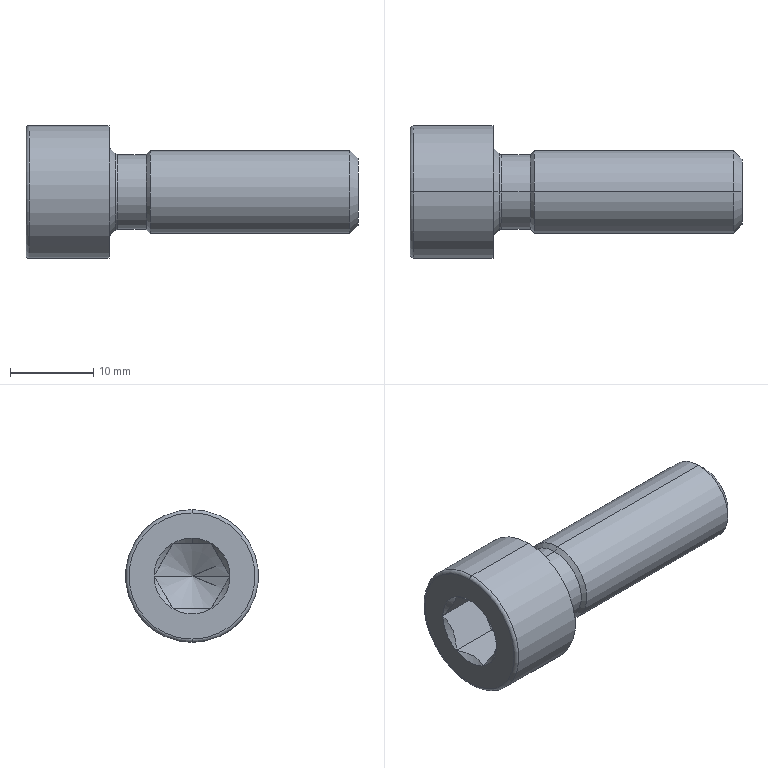Part | SolidWorks | features RevCut 2, Revolution 2, Chamfer 1, Cut 1, Fillet 1 | 1 solid | 42 faces | box 40 x 16 x 16 mm | volume 3907 mm3 | cone 15 | plane 15 | torus 6 | cylinder 6 | commonest cylinder face diameters 9.026 x2 10 x2 16 x2
STEP:
#1=CARTESIAN_POINT('',(40.,0.,-4.));
#2=VERTEX_POINT('',#1);
#3=CARTESIAN_POINT('',(40.,0.,4.));
#4=VERTEX_POINT('',#3);
#5=CARTESIAN_POINT('',(40.,0.,0.));
#6=DIRECTION('',(1.,0.,0.));
#7=DIRECTION('',(0.,0.,-1.));
#8=AXIS2_PLACEMENT_3D('',#5,#6,#7);
#9=CIRCLE('',#8,4.);
#10=EDGE_CURVE('',#2,#4,#9,.T.);
#11=ORIENTED_EDGE('',*,*,#10,.F.);
#12=CARTESIAN_POINT('',(39.,0.,-5.));
#13=VERTEX_POINT('',#12);
#14=CARTESIAN_POINT('',(40.,0.,-4.));
#15=DIRECTION('',(-0.7071,0.,-0.7071));
#16=VECTOR('',#15,1000.);
#17=LINE('',#14,#16);
#18=EDGE_CURVE('',#2,#13,#17,.T.);
#19=ORIENTED_EDGE('',*,*,#18,.T.);
#20=CARTESIAN_POINT('',(39.,0.,5.));
#21=VERTEX_POINT('',#20);
#22=CARTESIAN_POINT('',(39.,0.,0.));
#23=DIRECTION('',(-1.,0.,0.));
#24=DIRECTION('',(0.,0.,-1.));
#25=AXIS2_PLACEMENT_3D('',#22,#23,#24);
#26=CIRCLE('',#25,5.);
#27=EDGE_CURVE('',#21,#13,#26,.T.);
#28=ORIENTED_EDGE('',*,*,#27,.F.);
#29=CARTESIAN_POINT('',(40.,0.,4.));
#30=DIRECTION('',(-0.7071,0.,0.7071));
#31=VECTOR('',#30,1000.);
#32=LINE('',#29,#31);
#33=EDGE_CURVE('',#4,#21,#32,.T.);
#34=ORIENTED_EDGE('',*,*,#33,.F.);
#35=EDGE_LOOP('',(#11,#19,#28,#34));
#36=FACE_OUTER_BOUND('',#35,.T.);
#37=CARTESIAN_POINT('',(40.,0.,0.));
#38=DIRECTION('',(-1.,0.,0.));
#39=DIRECTION('',(0.,0.,1.));
#40=AXIS2_PLACEMENT_3D('',#37,#38,#39);
#41=CONICAL_SURFACE('',#40,4.,0.7854);
#42=ADVANCED_FACE('',(#36),#41,.T.);
#43=CARTESIAN_POINT('',(0.4,0.,-8.));
#44=VERTEX_POINT('',#43);
#45=CARTESIAN_POINT('',(0.4,0.,8.));
#46=VERTEX_POINT('',#45);
#47=CARTESIAN_POINT('',(0.4,0.,0.));
#48=DIRECTION('',(1.,0.,0.));
#49=DIRECTION('',(0.,0.,1.));
#50=AXIS2_PLACEMENT_3D('',#47,#48,#49);
#51=CIRCLE('',#50,8.);
#52=EDGE_CURVE('',#44,#46,#51,.T.);
#53=ORIENTED_EDGE('',*,*,#52,.F.);
#54=CARTESIAN_POINT('',(0.,0.,-7.6));
#55=VERTEX_POINT('',#54);
#56=CARTESIAN_POINT('',(0.4,0.,-7.6));
#57=DIRECTION('',(0.,1.,0.));
#58=DIRECTION('',(0.,0.,1.));
#59=AXIS2_PLACEMENT_3D('',#56,#57,#58);
#60=CIRCLE('',#59,0.4);
#61=EDGE_CURVE('',#44,#55,#60,.T.);
#62=ORIENTED_EDGE('',*,*,#61,.T.);
#63=CARTESIAN_POINT('',(0.,0.,7.6));
#64=VERTEX_POINT('',#63);
#65=CARTESIAN_POINT('',(0.,0.,0.));
#66=DIRECTION('',(-1.,0.,0.));
#67=DIRECTION('',(0.,0.,1.));
#68=AXIS2_PLACEMENT_3D('',#65,#66,#67);
#69=CIRCLE('',#68,7.6);
#70=EDGE_CURVE('',#64,#55,#69,.T.);
#71=ORIENTED_EDGE('',*,*,#70,.F.);
#72=CARTESIAN_POINT('',(0.4,0.,7.6));
#73=DIRECTION('',(0.,-1.,0.));
#74=DIRECTION('',(0.,0.,-1.));
#75=AXIS2_PLACEMENT_3D('',#72,#73,#74);
#76=CIRCLE('',#75,0.4);
#77=EDGE_CURVE('',#46,#64,#76,.T.);
#78=ORIENTED_EDGE('',*,*,#77,.F.);
#79=EDGE_LOOP('',(#53,#62,#71,#78));
#80=FACE_OUTER_BOUND('',#79,.T.);
#81=CARTESIAN_POINT('',(0.4,0.,0.));
#82=DIRECTION('',(-1.,0.,0.));
#83=DIRECTION('',(0.,0.,1.));
#84=AXIS2_PLACEMENT_3D('',#81,#82,#83);
#85=TOROIDAL_SURFACE('',#84,7.6,0.4);
#86=ADVANCED_FACE('',(#80),#85,.T.);
#87=CARTESIAN_POINT('',(8.641,0.,0.));
#88=VERTEX_POINT('',#87);
#89=CARTESIAN_POINT('',(6.,-4.575,0.));
#90=VERTEX_POINT('',#89);
#91=CARTESIAN_POINT('',(8.641,0.,0.));
#92=DIRECTION('',(-0.5,-0.866,0.));
#93=VECTOR('',#92,1000.);
#94=LINE('',#91,#93);
#95=EDGE_CURVE('',#88,#90,#94,.T.);
#96=ORIENTED_EDGE('',*,*,#95,.F.);
#97=CARTESIAN_POINT('',(6.,4.575,0.));
#98=VERTEX_POINT('',#97);
#99=CARTESIAN_POINT('',(8.641,0.,0.));
#100=DIRECTION('',(-0.5,0.866,0.));
#101=VECTOR('',#100,1000.);
#102=LINE('',#99,#101);
#103=EDGE_CURVE('',#88,#98,#102,.T.);
#104=ORIENTED_EDGE('',*,*,#103,.T.);
#105=CARTESIAN_POINT('',(6.,2.287,-3.962));
#106=VERTEX_POINT('',#105);
#107=CARTESIAN_POINT('',(6.,0.,0.));
#108=DIRECTION('',(-1.,0.,0.));
#109=DIRECTION('',(0.,-1.,0.));
#110=AXIS2_PLACEMENT_3D('',#107,#108,#109);
#111=CIRCLE('',#110,4.575);
#112=EDGE_CURVE('',#98,#106,#111,.T.);
#113=ORIENTED_EDGE('',*,*,#112,.T.);
#114=CARTESIAN_POINT('',(6.,-2.287,-3.962));
#115=VERTEX_POINT('',#114);
#116=CARTESIAN_POINT('',(6.,0.,0.));
#117=DIRECTION('',(-1.,0.,0.));
#118=DIRECTION('',(0.,-1.,0.));
#119=AXIS2_PLACEMENT_3D('',#116,#117,#118);
#120=CIRCLE('',#119,4.575);
#121=EDGE_CURVE('',#106,#115,#120,.T.);
#122=ORIENTED_EDGE('',*,*,#121,.T.);
#123=CARTESIAN_POINT('',(6.,0.,0.));
#124=DIRECTION('',(-1.,0.,0.));
#125=DIRECTION('',(0.,-1.,0.));
#126=AXIS2_PLACEMENT_3D('',#123,#124,#125);
#127=CIRCLE('',#126,4.575);
#128=EDGE_CURVE('',#115,#90,#127,.T.);
#129=ORIENTED_EDGE('',*,*,#128,.T.);
#130=EDGE_LOOP('',(#96,#104,#113,#122,#129));
#131=FACE_OUTER_BOUND('',#130,.T.);
#132=CARTESIAN_POINT('',(-991.359,0.,0.));
#133=DIRECTION('',(-1.,0.,0.));
#134=DIRECTION('',(0.,-1.,0.));
#135=AXIS2_PLACEMENT_3D('',#132,#133,#134);
#136=CONICAL_SURFACE('',#135,1732.051,1.047);
#137=ADVANCED_FACE('',(#131),#136,.F.);
#138=CARTESIAN_POINT('',(0.6129,0.,3.962));
#139=VERTEX_POINT('',#138);
#140=CARTESIAN_POINT('',(0.,2.288,3.962));
#141=VERTEX_POINT('',#140);
#142=CARTESIAN_POINT('',(0.6129,0.,3.962));
#143=CARTESIAN_POINT('',(0.6129,0.4023,3.962));
#144=CARTESIAN_POINT('',(0.5509,0.7939,3.962));
#145=CARTESIAN_POINT('',(0.387,1.369,3.962));
#146=CARTESIAN_POINT('',(0.3203,1.56,3.962));
#147=CARTESIAN_POINT('',(0.1711,1.93,3.962));
#148=CARTESIAN_POINT('',(0.08852,2.11,3.962));
#149=CARTESIAN_POINT('',(0.,2.288,3.962));
#150=B_SPLINE_CURVE_WITH_KNOTS('',3,(#142,#143,#144,#145,#146,#147,#148,#149),.UNSPECIFIED.,.F.,.F.,(4,2,2,4),(0.005342,0.006528,0.007121,0.007714),.UNSPECIFIED.);
#151=EDGE_CURVE('',#139,#141,#150,.T.);
#152=ORIENTED_EDGE('',*,*,#151,.F.);
#153=CARTESIAN_POINT('',(0.,0.,4.575));
#154=VERTEX_POINT('',#153);
#155=CARTESIAN_POINT('',(0.6129,0.,3.962));
#156=DIRECTION('',(-0.7071,0.,0.7071));
#157=VECTOR('',#156,1000.);
#158=LINE('',#155,#157);
#159=EDGE_CURVE('',#139,#154,#158,.T.);
#160=ORIENTED_EDGE('',*,*,#159,.T.);
#161=CARTESIAN_POINT('',(0.,0.,0.));
#162=DIRECTION('',(1.,0.,0.));
#163=DIRECTION('',(0.,0.,-1.));
#164=AXIS2_PLACEMENT_3D('',#161,#162,#163);
#165=CIRCLE('',#164,4.575);
#166=EDGE_CURVE('',#141,#154,#165,.T.);
#167=ORIENTED_EDGE('',*,*,#166,.F.);
#168=EDGE_LOOP('',(#152,#160,#167));
#169=FACE_OUTER_BOUND('',#168,.T.);
#170=CARTESIAN_POINT('',(0.6129,0.,0.));
#171=DIRECTION('',(-1.,0.,0.));
#172=DIRECTION('',(0.,0.,1.));
#173=AXIS2_PLACEMENT_3D('',#170,#171,#172);
#174=CONICAL_SURFACE('',#173,3.962,0.7854);
#175=ADVANCED_FACE('',(#169),#174,.F.);
#176=CARTESIAN_POINT('',(14.987,0.,-5.));
#177=VERTEX_POINT('',#176);
#178=CARTESIAN_POINT('',(14.987,0.,5.));
#179=VERTEX_POINT('',#178);
#180=CARTESIAN_POINT('',(14.987,0.,0.));
#181=DIRECTION('',(1.,0.,0.));
#182=DIRECTION('',(0.,0.,-1.));
#183=AXIS2_PLACEMENT_3D('',#180,#181,#182);
#184=CIRCLE('',#183,5.);
#185=EDGE_CURVE('',#177,#179,#184,.T.);
#186=ORIENTED_EDGE('',*,*,#185,.T.);
#187=CARTESIAN_POINT('',(0.,0.,5.));
#188=DIRECTION('',(1.,0.,0.));
#189=VECTOR('',#188,1000.);
#190=LINE('',#187,#189);
#191=EDGE_CURVE('',#179,#21,#190,.T.);
#192=ORIENTED_EDGE('',*,*,#191,.T.);
#193=ORIENTED_EDGE('',*,*,#27,.T.);
#194=CARTESIAN_POINT('',(0.,0.,-5.));
#195=DIRECTION('',(1.,0.,0.));
#196=VECTOR('',#195,1000.);
#197=LINE('',#194,#196);
#198=EDGE_CURVE('',#177,#13,#197,.T.);
#199=ORIENTED_EDGE('',*,*,#198,.F.);
#200=EDGE_LOOP('',(#186,#192,#193,#199));
#201=FACE_OUTER_BOUND('',#200,.T.);
#202=CARTESIAN_POINT('',(0.,0.,0.));
#203=DIRECTION('',(1.,0.,0.));
#204=DIRECTION('',(0.,0.,-1.));
#205=AXIS2_PLACEMENT_3D('',#202,#203,#204);
#206=CYLINDRICAL_SURFACE('',#205,5.);
#207=ADVANCED_FACE('',(#201),#206,.T.);
#208=CARTESIAN_POINT('',(14.5,0.,-4.513));
#209=VERTEX_POINT('',#208);
#210=CARTESIAN_POINT('',(14.5,0.,4.513));
#211=VERTEX_POINT('',#210);
#212=CARTESIAN_POINT('',(14.5,0.,0.));
#213=DIRECTION('',(1.,0.,0.));
#214=DIRECTION('',(0.,0.,-1.));
#215=AXIS2_PLACEMENT_3D('',#212,#213,#214);
#216=CIRCLE('',#215,4.513);
#217=EDGE_CURVE('',#209,#211,#216,.T.);
#218=ORIENTED_EDGE('',*,*,#217,.T.);
#219=CARTESIAN_POINT('',(14.987,0.,5.));
#220=DIRECTION('',(0.7071,0.,0.7071));
#221=VECTOR('',#220,1000.);
#222=LINE('',#219,#221);
#223=EDGE_CURVE('',#211,#179,#222,.T.);
#224=ORIENTED_EDGE('',*,*,#223,.T.);
#225=ORIENTED_EDGE('',*,*,#185,.F.);
#226=CARTESIAN_POINT('',(14.987,0.,-5.));
#227=DIRECTION('',(0.7071,0.,-0.7071));
#228=VECTOR('',#227,1000.);
#229=LINE('',#226,#228);
#230=EDGE_CURVE('',#209,#177,#229,.T.);
#231=ORIENTED_EDGE('',*,*,#230,.F.);
#232=EDGE_LOOP('',(#218,#224,#225,#231));
#233=FACE_OUTER_BOUND('',#232,.T.);
#234=CARTESIAN_POINT('',(14.987,0.,0.));
#235=DIRECTION('',(1.,0.,0.));
#236=DIRECTION('',(0.,0.,-1.));
#237=AXIS2_PLACEMENT_3D('',#234,#235,#236);
#238=CONICAL_SURFACE('',#237,5.,0.7854);
#239=ADVANCED_FACE('',(#233),#238,.T.);
#240=CARTESIAN_POINT('',(11.02,0.,-4.513));
#241=VERTEX_POINT('',#240);
#242=CARTESIAN_POINT('',(11.02,0.,4.513));
#243=VERTEX_POINT('',#242);
#244=CARTESIAN_POINT('',(11.02,0.,0.));
#245=DIRECTION('',(1.,0.,0.));
#246=DIRECTION('',(0.,0.,-1.));
#247=AXIS2_PLACEMENT_3D('',#244,#245,#246);
#248=CIRCLE('',#247,4.513);
#249=EDGE_CURVE('',#241,#243,#248,.T.);
#250=ORIENTED_EDGE('',*,*,#249,.T.);
#251=CARTESIAN_POINT('',(0.,0.,4.513));
#252=DIRECTION('',(1.,0.,0.));
#253=VECTOR('',#252,1000.);
#254=LINE('',#251,#253);
#255=EDGE_CURVE('',#243,#211,#254,.T.);
#256=ORIENTED_EDGE('',*,*,#255,.T.);
#257=ORIENTED_EDGE('',*,*,#217,.F.);
#258=CARTESIAN_POINT('',(0.,0.,-4.513));
#259=DIRECTION('',(1.,0.,0.));
#260=VECTOR('',#259,1000.);
#261=LINE('',#258,#260);
#262=EDGE_CURVE('',#241,#209,#261,.T.);
#263=ORIENTED_EDGE('',*,*,#262,.F.);
#264=EDGE_LOOP('',(#250,#256,#257,#263));
#265=FACE_OUTER_BOUND('',#264,.T.);
#266=CARTESIAN_POINT('',(0.,0.,0.));
#267=DIRECTION('',(1.,0.,0.));
#268=DIRECTION('',(0.,0.,-1.));
#269=AXIS2_PLACEMENT_3D('',#266,#267,#268);
#270=CYLINDRICAL_SURFACE('',#269,4.513);
#271=ADVANCED_FACE('',(#265),#270,.T.);
#272=CARTESIAN_POINT('',(11.02,0.,0.));
#273=DIRECTION('',(1.,0.,0.));
#274=DIRECTION('',(0.,0.,-1.));
#275=AXIS2_PLACEMENT_3D('',#272,#273,#274);
#276=CIRCLE('',#275,4.513);
#277=EDGE_CURVE('',#243,#241,#276,.T.);
#278=ORIENTED_EDGE('',*,*,#277,.F.);
#279=CARTESIAN_POINT('',(10.723,0.,4.645));
#280=VERTEX_POINT('',#279);
#281=CARTESIAN_POINT('',(11.02,0.,4.913));
#282=DIRECTION('',(0.,1.,0.));
#283=DIRECTION('',(0.,0.,1.));
#284=AXIS2_PLACEMENT_3D('',#281,#282,#283);
#285=CIRCLE('',#284,0.4);
#286=EDGE_CURVE('',#243,#280,#285,.T.);
#287=ORIENTED_EDGE('',*,*,#286,.T.);
#288=CARTESIAN_POINT('',(10.723,0.,-4.645));
#289=VERTEX_POINT('',#288);
#290=CARTESIAN_POINT('',(10.723,0.,0.));
#291=DIRECTION('',(1.,0.,0.));
#292=DIRECTION('',(0.,0.,-1.));
#293=AXIS2_PLACEMENT_3D('',#290,#291,#292);
#294=CIRCLE('',#293,4.645);
#295=EDGE_CURVE('',#280,#289,#294,.T.);
#296=ORIENTED_EDGE('',*,*,#295,.T.);
#297=CARTESIAN_POINT('',(11.02,0.,-4.913));
#298=DIRECTION('',(0.,-1.,0.));
#299=DIRECTION('',(0.,0.,-1.));
#300=AXIS2_PLACEMENT_3D('',#297,#298,#299);
#301=CIRCLE('',#300,0.4);
#302=EDGE_CURVE('',#241,#289,#301,.T.);
#303=ORIENTED_EDGE('',*,*,#302,.F.);
#304=EDGE_LOOP('',(#278,#287,#296,#303));
#305=FACE_OUTER_BOUND('',#304,.T.);
#306=CARTESIAN_POINT('',(11.02,0.,0.));
#307=DIRECTION('',(1.,0.,0.));
#308=DIRECTION('',(0.,0.,-1.));
#309=AXIS2_PLACEMENT_3D('',#306,#307,#308);
#310=TOROIDAL_SURFACE('',#309,4.913,0.4);
#311=ADVANCED_FACE('',(#305),#310,.F.);
#312=CARTESIAN_POINT('',(10.723,0.,0.));
#313=DIRECTION('',(1.,0.,0.));
#314=DIRECTION('',(0.,0.,-1.));
#315=AXIS2_PLACEMENT_3D('',#312,#313,#314);
#316=CIRCLE('',#315,4.645);
#317=EDGE_CURVE('',#289,#280,#316,.T.);
#318=ORIENTED_EDGE('',*,*,#317,.F.);
#319=CARTESIAN_POINT('',(10.103,0.,-5.332));
#320=VERTEX_POINT('',#319);
#321=CARTESIAN_POINT('',(10.723,0.,-4.645));
#322=DIRECTION('',(-0.67,0.,-0.7424));
#323=VECTOR('',#322,1000.);
#324=LINE('',#321,#323);
#325=EDGE_CURVE('',#289,#320,#324,.T.);
#326=ORIENTED_EDGE('',*,*,#325,.T.);
#327=CARTESIAN_POINT('',(10.103,0.,5.332));
#328=VERTEX_POINT('',#327);
#329=CARTESIAN_POINT('',(10.103,0.,0.));
#330=DIRECTION('',(1.,0.,0.));
#331=DIRECTION('',(0.,0.,-1.));
#332=AXIS2_PLACEMENT_3D('',#329,#330,#331);
#333=CIRCLE('',#332,5.332);
#334=EDGE_CURVE('',#320,#328,#333,.T.);
#335=ORIENTED_EDGE('',*,*,#334,.T.);
#336=CARTESIAN_POINT('',(10.723,0.,4.645));
#337=DIRECTION('',(-0.67,0.,0.7424));
#338=VECTOR('',#337,1000.);
#339=LINE('',#336,#338);
#340=EDGE_CURVE('',#280,#328,#339,.T.);
#341=ORIENTED_EDGE('',*,*,#340,.F.);
#342=EDGE_LOOP('',(#318,#326,#335,#341));
#343=FACE_OUTER_BOUND('',#342,.T.);
#344=CARTESIAN_POINT('',(10.723,0.,0.));
#345=DIRECTION('',(-1.,0.,0.));
#346=DIRECTION('',(0.,0.,1.));
#347=AXIS2_PLACEMENT_3D('',#344,#345,#346);
#348=CONICAL_SURFACE('',#347,4.645,0.8366);
#349=ADVANCED_FACE('',(#343),#348,.T.);
#350=CARTESIAN_POINT('',(10.103,0.,0.));
#351=DIRECTION('',(1.,0.,0.));
#352=DIRECTION('',(0.,0.,-1.));
#353=AXIS2_PLACEMENT_3D('',#350,#351,#352);
#354=CIRCLE('',#353,5.332);
#355=EDGE_CURVE('',#328,#320,#354,.T.);
#356=ORIENTED_EDGE('',*,*,#355,.F.);
#357=CARTESIAN_POINT('',(10.,0.,5.6));
#358=VERTEX_POINT('',#357);
#359=CARTESIAN_POINT('',(10.4,0.,5.6));
#360=DIRECTION('',(0.,1.,0.));
#361=DIRECTION('',(0.,0.,1.));
#362=AXIS2_PLACEMENT_3D('',#359,#360,#361);
#363=CIRCLE('',#362,0.4);
#364=EDGE_CURVE('',#328,#358,#363,.T.);
#365=ORIENTED_EDGE('',*,*,#364,.T.);
#366=CARTESIAN_POINT('',(10.,0.,-5.6));
#367=VERTEX_POINT('',#366);
#368=CARTESIAN_POINT('',(10.,0.,0.));
#369=DIRECTION('',(1.,0.,0.));
#370=DIRECTION('',(0.,0.,-1.));
#371=AXIS2_PLACEMENT_3D('',#368,#369,#370);
#372=CIRCLE('',#371,5.6);
#373=EDGE_CURVE('',#358,#367,#372,.T.);
#374=ORIENTED_EDGE('',*,*,#373,.T.);
#375=CARTESIAN_POINT('',(10.4,0.,-5.6));
#376=DIRECTION('',(0.,-1.,0.));
#377=DIRECTION('',(0.,0.,-1.));
#378=AXIS2_PLACEMENT_3D('',#375,#376,#377);
#379=CIRCLE('',#378,0.4);
#380=EDGE_CURVE('',#320,#367,#379,.T.);
#381=ORIENTED_EDGE('',*,*,#380,.F.);
#382=EDGE_LOOP('',(#356,#365,#374,#381));
#383=FACE_OUTER_BOUND('',#382,.T.);
#384=CARTESIAN_POINT('',(10.4,0.,0.));
#385=DIRECTION('',(1.,0.,0.));
#386=DIRECTION('',(0.,0.,-1.));
#387=AXIS2_PLACEMENT_3D('',#384,#385,#386);
#388=TOROIDAL_SURFACE('',#387,5.6,0.4);
#389=ADVANCED_FACE('',(#383),#388,.F.);
#390=ORIENTED_EDGE('',*,*,#52,.T.);
#391=CARTESIAN_POINT('',(10.,0.,8.));
#392=VERTEX_POINT('',#391);
#393=CARTESIAN_POINT('',(0.,0.,8.));
#394=DIRECTION('',(1.,0.,0.));
#395=VECTOR('',#394,1000.);
#396=LINE('',#393,#395);
#397=EDGE_CURVE('',#46,#392,#396,.T.);
#398=ORIENTED_EDGE('',*,*,#397,.T.);
#399=CARTESIAN_POINT('',(10.,0.,-8.));
#400=VERTEX_POINT('',#399);
#401=CARTESIAN_POINT('',(10.,0.,0.));
#402=DIRECTION('',(1.,0.,0.));
#403=DIRECTION('',(0.,0.,-1.));
#404=AXIS2_PLACEMENT_3D('',#401,#402,#403);
#405=CIRCLE('',#404,8.);
#406=EDGE_CURVE('',#400,#392,#405,.T.);
#407=ORIENTED_EDGE('',*,*,#406,.F.);
#408=CARTESIAN_POINT('',(0.,0.,-8.));
#409=DIRECTION('',(1.,0.,0.));
#410=VECTOR('',#409,1000.);
#411=LINE('',#408,#410);
#412=EDGE_CURVE('',#44,#400,#411,.T.);
#413=ORIENTED_EDGE('',*,*,#412,.F.);
#414=EDGE_LOOP('',(#390,#398,#407,#413));
#415=FACE_OUTER_BOUND('',#414,.T.);
#416=CARTESIAN_POINT('',(0.,0.,0.));
#417=DIRECTION('',(1.,0.,0.));
#418=DIRECTION('',(0.,0.,-1.));
#419=AXIS2_PLACEMENT_3D('',#416,#417,#418);
#420=CYLINDRICAL_SURFACE('',#419,8.);
#421=ADVANCED_FACE('',(#415),#420,.T.);
#422=ORIENTED_EDGE('',*,*,#70,.T.);
#423=CARTESIAN_POINT('',(0.,0.,0.));
#424=DIRECTION('',(-1.,0.,0.));
#425=DIRECTION('',(0.,0.,1.));
#426=AXIS2_PLACEMENT_3D('',#423,#424,#425);
#427=CIRCLE('',#426,7.6);
#428=EDGE_CURVE('',#55,#64,#427,.T.);
#429=ORIENTED_EDGE('',*,*,#428,.T.);
#430=EDGE_LOOP('',(#422,#429));
#431=FACE_OUTER_BOUND('',#430,.T.);
#432=CARTESIAN_POINT('',(0.,4.575,0.));
#433=VERTEX_POINT('',#432);
#434=CARTESIAN_POINT('',(0.,0.,0.));
#435=DIRECTION('',(1.,0.,0.));
#436=DIRECTION('',(0.,0.,-1.));
#437=AXIS2_PLACEMENT_3D('',#434,#435,#436);
#438=CIRCLE('',#437,4.575);
#439=EDGE_CURVE('',#433,#141,#438,.T.);
#440=ORIENTED_EDGE('',*,*,#439,.T.);
#441=ORIENTED_EDGE('',*,*,#166,.T.);
#442=CARTESIAN_POINT('',(0.,-2.288,3.962));
#443=VERTEX_POINT('',#442);
#444=CARTESIAN_POINT('',(0.,0.,0.));
#445=DIRECTION('',(1.,0.,0.));
#446=DIRECTION('',(0.,0.,-1.));
#447=AXIS2_PLACEMENT_3D('',#444,#445,#446);
#448=CIRCLE('',#447,4.575);
#449=EDGE_CURVE('',#154,#443,#448,.T.);
#450=ORIENTED_EDGE('',*,*,#449,.T.);
#451=CARTESIAN_POINT('',(0.,-4.575,0.));
#452=VERTEX_POINT('',#451);
#453=CARTESIAN_POINT('',(0.,0.,0.));
#454=DIRECTION('',(1.,0.,0.));
#455=DIRECTION('',(0.,0.,-1.));
#456=AXIS2_PLACEMENT_3D('',#453,#454,#455);
#457=CIRCLE('',#456,4.575);
#458=EDGE_CURVE('',#443,#452,#457,.T.);
#459=ORIENTED_EDGE('',*,*,#458,.T.);
#460=CARTESIAN_POINT('',(0.,-2.288,-3.962));
#461=VERTEX_POINT('',#460);
#462=CARTESIAN_POINT('',(0.,0.,0.));
#463=DIRECTION('',(1.,0.,0.));
#464=DIRECTION('',(0.,0.,-1.));
#465=AXIS2_PLACEMENT_3D('',#462,#463,#464);
#466=CIRCLE('',#465,4.575);
#467=EDGE_CURVE('',#452,#461,#466,.T.);
#468=ORIENTED_EDGE('',*,*,#467,.T.);
#469=CARTESIAN_POINT('',(0.,2.288,-3.962));
#470=VERTEX_POINT('',#469);
#471=CARTESIAN_POINT('',(0.,0.,0.));
#472=DIRECTION('',(1.,0.,0.));
#473=DIRECTION('',(0.,0.,-1.));
#474=AXIS2_PLACEMENT_3D('',#471,#472,#473);
#475=CIRCLE('',#474,4.575);
#476=EDGE_CURVE('',#461,#470,#475,.T.);
#477=ORIENTED_EDGE('',*,*,#476,.T.);
#478=CARTESIAN_POINT('',(0.,0.,0.));
#479=DIRECTION('',(1.,0.,0.));
#480=DIRECTION('',(0.,0.,-1.));
#481=AXIS2_PLACEMENT_3D('',#478,#479,#480);
#482=CIRCLE('',#481,4.575);
#483=EDGE_CURVE('',#470,#433,#482,.T.);
#484=ORIENTED_EDGE('',*,*,#483,.T.);
#485=EDGE_LOOP('',(#440,#441,#450,#459,#468,#477,#484));
#486=FACE_BOUND('',#485,.T.);
#487=CARTESIAN_POINT('',(0.,0.,0.));
#488=DIRECTION('',(-1.,0.,0.));
#489=DIRECTION('',(0.,0.,1.));
#490=AXIS2_PLACEMENT_3D('',#487,#488,#489);
#491=PLANE('',#490);
#492=ADVANCED_FACE('',(#431,#486),#491,.T.);
#493=ORIENTED_EDGE('',*,*,#397,.F.);
#494=CARTESIAN_POINT('',(0.4,0.,0.));
#495=DIRECTION('',(1.,0.,0.));
#496=DIRECTION('',(0.,0.,1.));
#497=AXIS2_PLACEMENT_3D('',#494,#495,#496);
#498=CIRCLE('',#497,8.);
#499=EDGE_CURVE('',#46,#44,#498,.T.);
#500=ORIENTED_EDGE('',*,*,#499,.T.);
#501=ORIENTED_EDGE('',*,*,#412,.T.);
#502=CARTESIAN_POINT('',(10.,0.,0.));
#503=DIRECTION('',(1.,0.,0.));
#504=DIRECTION('',(0.,0.,-1.));
#505=AXIS2_PLACEMENT_3D('',#502,#503,#504);
#506=CIRCLE('',#505,8.);
#507=EDGE_CURVE('',#392,#400,#506,.T.);
#508=ORIENTED_EDGE('',*,*,#507,.F.);
#509=EDGE_LOOP('',(#493,#500,#501,#508));
#510=FACE_OUTER_BOUND('',#509,.T.);
#511=CARTESIAN_POINT('',(0.,0.,0.));
#512=DIRECTION('',(1.,0.,0.));
#513=DIRECTION('',(0.,0.,-1.));
#514=AXIS2_PLACEMENT_3D('',#511,#512,#513);
#515=CYLINDRICAL_SURFACE('',#514,8.);
#516=ADVANCED_FACE('',(#510),#515,.T.);
#517=ORIENTED_EDGE('',*,*,#406,.T.);
#518=ORIENTED_EDGE('',*,*,#507,.T.);
#519=EDGE_LOOP('',(#517,#518));
#520=FACE_OUTER_BOUND('',#519,.T.);
#521=CARTESIAN_POINT('',(10.,0.,0.));
#522=DIRECTION('',(1.,0.,0.));
#523=DIRECTION('',(0.,0.,-1.));
#524=AXIS2_PLACEMENT_3D('',#521,#522,#523);
#525=CIRCLE('',#524,5.6);
#526=EDGE_CURVE('',#367,#358,#525,.T.);
#527=ORIENTED_EDGE('',*,*,#526,.F.);
#528=ORIENTED_EDGE('',*,*,#373,.F.);
#529=EDGE_LOOP('',(#527,#528));
#530=FACE_BOUND('',#529,.T.);
#531=CARTESIAN_POINT('',(10.,8.,0.));
#532=DIRECTION('',(1.,0.,0.));
#533=DIRECTION('',(0.,0.,-1.));
#534=AXIS2_PLACEMENT_3D('',#531,#532,#533);
#535=PLANE('',#534);
#536=ADVANCED_FACE('',(#520,#530),#535,.T.);
#537=ORIENTED_EDGE('',*,*,#364,.F.);
#538=ORIENTED_EDGE('',*,*,#334,.F.);
#539=ORIENTED_EDGE('',*,*,#380,.T.);
#540=ORIENTED_EDGE('',*,*,#526,.T.);
#541=EDGE_LOOP('',(#537,#538,#539,#540));
#542=FACE_OUTER_BOUND('',#541,.T.);
#543=CARTESIAN_POINT('',(10.4,0.,0.));
#544=DIRECTION('',(1.,0.,0.));
#545=DIRECTION('',(0.,0.,-1.));
#546=AXIS2_PLACEMENT_3D('',#543,#544,#545);
#547=TOROIDAL_SURFACE('',#546,5.6,0.4);
#548=ADVANCED_FACE('',(#542),#547,.F.);
#549=ORIENTED_EDGE('',*,*,#325,.F.);
#550=ORIENTED_EDGE('',*,*,#295,.F.);
#551=ORIENTED_EDGE('',*,*,#340,.T.);
#552=ORIENTED_EDGE('',*,*,#355,.T.);
#553=EDGE_LOOP('',(#549,#550,#551,#552));
#554=FACE_OUTER_BOUND('',#553,.T.);
#555=CARTESIAN_POINT('',(10.723,0.,0.));
#556=DIRECTION('',(-1.,0.,0.));
#557=DIRECTION('',(0.,0.,1.));
#558=AXIS2_PLACEMENT_3D('',#555,#556,#557);
#559=CONICAL_SURFACE('',#558,4.645,0.8366);
#560=ADVANCED_FACE('',(#554),#559,.T.);
#561=ORIENTED_EDGE('',*,*,#286,.F.);
#562=ORIENTED_EDGE('',*,*,#249,.F.);
#563=ORIENTED_EDGE('',*,*,#302,.T.);
#564=ORIENTED_EDGE('',*,*,#317,.T.);
#565=EDGE_LOOP('',(#561,#562,#563,#564));
#566=FACE_OUTER_BOUND('',#565,.T.);
#567=CARTESIAN_POINT('',(11.02,0.,0.));
#568=DIRECTION('',(1.,0.,0.));
#569=DIRECTION('',(0.,0.,-1.));
#570=AXIS2_PLACEMENT_3D('',#567,#568,#569);
#571=TOROIDAL_SURFACE('',#570,4.913,0.4);
#572=ADVANCED_FACE('',(#566),#571,.F.);
#573=ORIENTED_EDGE('',*,*,#255,.F.);
#574=ORIENTED_EDGE('',*,*,#277,.T.);
#575=ORIENTED_EDGE('',*,*,#262,.T.);
#576=CARTESIAN_POINT('',(14.5,0.,0.));
#577=DIRECTION('',(1.,0.,0.));
#578=DIRECTION('',(0.,0.,-1.));
#579=AXIS2_PLACEMENT_3D('',#576,#577,#578);
#580=CIRCLE('',#579,4.513);
#581=EDGE_CURVE('',#211,#209,#580,.T.);
#582=ORIENTED_EDGE('',*,*,#581,.F.);
#583=EDGE_LOOP('',(#573,#574,#575,#582));
#584=FACE_OUTER_BOUND('',#583,.T.);
#585=CARTESIAN_POINT('',(0.,0.,0.));
#586=DIRECTION('',(1.,0.,0.));
#587=DIRECTION('',(0.,0.,-1.));
#588=AXIS2_PLACEMENT_3D('',#585,#586,#587);
#589=CYLINDRICAL_SURFACE('',#588,4.513);
#590=ADVANCED_FACE('',(#584),#589,.T.);
#591=ORIENTED_EDGE('',*,*,#223,.F.);
#592=ORIENTED_EDGE('',*,*,#581,.T.);
#593=ORIENTED_EDGE('',*,*,#230,.T.);
#594=CARTESIAN_POINT('',(14.987,0.,0.));
#595=DIRECTION('',(1.,0.,0.));
#596=DIRECTION('',(0.,0.,-1.));
#597=AXIS2_PLACEMENT_3D('',#594,#595,#596);
#598=CIRCLE('',#597,5.);
#599=EDGE_CURVE('',#179,#177,#598,.T.);
#600=ORIENTED_EDGE('',*,*,#599,.F.);
#601=EDGE_LOOP('',(#591,#592,#593,#600));
#602=FACE_OUTER_BOUND('',#601,.T.);
#603=CARTESIAN_POINT('',(14.987,0.,0.));
#604=DIRECTION('',(1.,0.,0.));
#605=DIRECTION('',(0.,0.,-1.));
#606=AXIS2_PLACEMENT_3D('',#603,#604,#605);
#607=CONICAL_SURFACE('',#606,5.,0.7854);
#608=ADVANCED_FACE('',(#602),#607,.T.);
#609=ORIENTED_EDGE('',*,*,#191,.F.);
#610=ORIENTED_EDGE('',*,*,#599,.T.);
#611=ORIENTED_EDGE('',*,*,#198,.T.);
#612=CARTESIAN_POINT('',(39.,0.,0.));
#613=DIRECTION('',(-1.,0.,0.));
#614=DIRECTION('',(0.,0.,-1.));
#615=AXIS2_PLACEMENT_3D('',#612,#613,#614);
#616=CIRCLE('',#615,5.);
#617=EDGE_CURVE('',#13,#21,#616,.T.);
#618=ORIENTED_EDGE('',*,*,#617,.T.);
#619=EDGE_LOOP('',(#609,#610,#611,#618));
#620=FACE_OUTER_BOUND('',#619,.T.);
#621=CARTESIAN_POINT('',(0.,0.,0.));
#622=DIRECTION('',(1.,0.,0.));
#623=DIRECTION('',(0.,0.,-1.));
#624=AXIS2_PLACEMENT_3D('',#621,#622,#623);
#625=CYLINDRICAL_SURFACE('',#624,5.);
#626=ADVANCED_FACE('',(#620),#625,.T.);
#627=CARTESIAN_POINT('',(40.,0.,0.));
#628=DIRECTION('',(1.,0.,0.));
#629=DIRECTION('',(0.,0.,-1.));
#630=AXIS2_PLACEMENT_3D('',#627,#628,#629);
#631=CIRCLE('',#630,4.);
#632=EDGE_CURVE('',#4,#2,#631,.T.);
#633=ORIENTED_EDGE('',*,*,#632,.T.);
#634=ORIENTED_EDGE('',*,*,#10,.T.);
#635=EDGE_LOOP('',(#633,#634));
#636=FACE_OUTER_BOUND('',#635,.T.);
#637=CARTESIAN_POINT('',(40.,5.,0.));
#638=DIRECTION('',(1.,0.,0.));
#639=DIRECTION('',(0.,0.,-1.));
#640=AXIS2_PLACEMENT_3D('',#637,#638,#639);
#641=PLANE('',#640);
#642=ADVANCED_FACE('',(#636),#641,.T.);
#643=ORIENTED_EDGE('',*,*,#159,.F.);
#644=CARTESIAN_POINT('',(0.,-2.288,3.962));
#645=CARTESIAN_POINT('',(0.1774,-1.933,3.962));
#646=CARTESIAN_POINT('',(0.3328,-1.559,3.962));
#647=CARTESIAN_POINT('',(0.4959,-0.987,3.962));
#648=CARTESIAN_POINT('',(0.5389,-0.7937,3.962));
#649=CARTESIAN_POINT('',(0.5974,-0.4013,3.962));
#650=CARTESIAN_POINT('',(0.6129,-0.2009,3.962));
#651=CARTESIAN_POINT('',(0.6129,0.,3.962));
#652=B_SPLINE_CURVE_WITH_KNOTS('',3,(#644,#645,#646,#647,#648,#649,#650,#651),.UNSPECIFIED.,.F.,.F.,(4,2,2,4),(0.002971,0.004156,0.004749,0.005342),.UNSPECIFIED.);
#653=EDGE_CURVE('',#443,#139,#652,.T.);
#654=ORIENTED_EDGE('',*,*,#653,.F.);
#655=ORIENTED_EDGE('',*,*,#449,.F.);
#656=EDGE_LOOP('',(#643,#654,#655));
#657=FACE_OUTER_BOUND('',#656,.T.);
#658=CARTESIAN_POINT('',(0.6129,0.,0.));
#659=DIRECTION('',(-1.,0.,0.));
#660=DIRECTION('',(0.,0.,1.));
#661=AXIS2_PLACEMENT_3D('',#658,#659,#660);
#662=CONICAL_SURFACE('',#661,3.962,0.7854);
#663=ADVANCED_FACE('',(#657),#662,.F.);
#664=CARTESIAN_POINT('',(0.,2.288,3.962));
#665=CARTESIAN_POINT('',(0.1787,2.466,3.653));
#666=CARTESIAN_POINT('',(0.3307,2.649,3.336));
#667=CARTESIAN_POINT('',(0.4935,2.933,2.844));
#668=CARTESIAN_POINT('',(0.5369,3.029,2.677));
#669=CARTESIAN_POINT('',(0.5965,3.226,2.337));
#670=CARTESIAN_POINT('',(0.6125,3.327,2.161));
#671=CARTESIAN_POINT('',(0.6138,3.627,1.642));
#672=CARTESIAN_POINT('',(0.5533,3.823,1.302));
#673=CARTESIAN_POINT('',(0.3339,4.21,0.632));
#674=CARTESIAN_POINT('',(0.1798,4.395,0.3114));
#675=CARTESIAN_POINT('',(0.,4.575,0.));
#676=B_SPLINE_CURVE_WITH_KNOTS('',3,(#664,#665,#666,#667,#668,#669,#670,#671,#672,#673,#674,#675),.UNSPECIFIED.,.F.,.F.,(4,2,2,2,2,4),(0.000000254,0.001182,0.001772,0.002363,0.003545,0.004726),.UNSPECIFIED.);
#677=EDGE_CURVE('',#141,#433,#676,.T.);
#678=ORIENTED_EDGE('',*,*,#677,.F.);
#679=ORIENTED_EDGE('',*,*,#439,.F.);
#680=EDGE_LOOP('',(#678,#679));
#681=FACE_OUTER_BOUND('',#680,.T.);
#682=CARTESIAN_POINT('',(0.6129,0.,0.));
#683=DIRECTION('',(-1.,0.,0.));
#684=DIRECTION('',(0.,0.,1.));
#685=AXIS2_PLACEMENT_3D('',#682,#683,#684);
#686=CONICAL_SURFACE('',#685,3.962,0.7854);
#687=ADVANCED_FACE('',(#681),#686,.F.);
#688=CARTESIAN_POINT('',(0.,4.575,0.));
#689=CARTESIAN_POINT('',(0.1787,4.396,-0.3096));
#690=CARTESIAN_POINT('',(0.3307,4.214,-0.6261));
#691=CARTESIAN_POINT('',(0.4935,3.93,-1.118));
#692=CARTESIAN_POINT('',(0.5369,3.833,-1.285));
#693=CARTESIAN_POINT('',(0.5965,3.637,-1.625));
#694=CARTESIAN_POINT('',(0.6125,3.535,-1.801));
#695=CARTESIAN_POINT('',(0.6138,3.236,-2.32));
#696=CARTESIAN_POINT('',(0.5533,3.039,-2.66));
#697=CARTESIAN_POINT('',(0.3339,2.652,-3.33));
#698=CARTESIAN_POINT('',(0.1798,2.467,-3.651));
#699=CARTESIAN_POINT('',(0.,2.288,-3.962));
#700=B_SPLINE_CURVE_WITH_KNOTS('',3,(#688,#689,#690,#691,#692,#693,#694,#695,#696,#697,#698,#699),.UNSPECIFIED.,.F.,.F.,(4,2,2,2,2,4),(0.000000254,0.001182,0.001772,0.002363,0.003545,0.004726),.UNSPECIFIED.);
#701=EDGE_CURVE('',#433,#470,#700,.T.);
#702=ORIENTED_EDGE('',*,*,#701,.F.);
#703=ORIENTED_EDGE('',*,*,#483,.F.);
#704=EDGE_LOOP('',(#702,#703));
#705=FACE_OUTER_BOUND('',#704,.T.);
#706=CARTESIAN_POINT('',(0.6129,0.,0.));
#707=DIRECTION('',(-1.,0.,0.));
#708=DIRECTION('',(0.,0.,1.));
#709=AXIS2_PLACEMENT_3D('',#706,#707,#708);
#710=CONICAL_SURFACE('',#709,3.962,0.7854);
#711=ADVANCED_FACE('',(#705),#710,.F.);
#712=ORIENTED_EDGE('',*,*,#476,.F.);
#713=CARTESIAN_POINT('',(0.,2.288,-3.962));
#714=CARTESIAN_POINT('',(0.08848,2.111,-3.962));
#715=CARTESIAN_POINT('',(0.171,1.93,-3.962));
#716=CARTESIAN_POINT('',(0.3202,1.56,-3.962));
#717=CARTESIAN_POINT('',(0.3869,1.37,-3.962));
#718=CARTESIAN_POINT('',(0.5508,0.7947,-3.962));
#719=CARTESIAN_POINT('',(0.6128,0.4032,-3.962));
#720=CARTESIAN_POINT('',(0.613,-0.1999,-3.962));
#721=CARTESIAN_POINT('',(0.5975,-0.4004,-3.962));
#722=CARTESIAN_POINT('',(0.539,-0.793,-3.962));
#723=CARTESIAN_POINT('',(0.4961,-0.9864,-3.962));
#724=CARTESIAN_POINT('',(0.333,-1.559,-3.962));
#725=CARTESIAN_POINT('',(0.1775,-1.933,-3.962));
#726=CARTESIAN_POINT('',(0.,-2.288,-3.962));
#727=B_SPLINE_CURVE_WITH_KNOTS('',3,(#713,#714,#715,#716,#717,#718,#719,#720,#721,#722,#723,#724,#725,#726),.UNSPECIFIED.,.F.,.F.,(4,2,2,2,2,2,4),(0.002432,0.003025,0.003617,0.004802,0.005395,0.005987,0.007172),.UNSPECIFIED.);
#728=EDGE_CURVE('',#470,#461,#727,.T.);
#729=ORIENTED_EDGE('',*,*,#728,.F.);
#730=EDGE_LOOP('',(#712,#729));
#731=FACE_OUTER_BOUND('',#730,.T.);
#732=CARTESIAN_POINT('',(0.6129,0.,0.));
#733=DIRECTION('',(-1.,0.,0.));
#734=DIRECTION('',(0.,0.,1.));
#735=AXIS2_PLACEMENT_3D('',#732,#733,#734);
#736=CONICAL_SURFACE('',#735,3.962,0.7854);
#737=ADVANCED_FACE('',(#731),#736,.F.);
#738=ORIENTED_EDGE('',*,*,#467,.F.);
#739=CARTESIAN_POINT('',(0.,-2.288,-3.962));
#740=CARTESIAN_POINT('',(0.1787,-2.466,-3.653));
#741=CARTESIAN_POINT('',(0.3307,-2.649,-3.336));
#742=CARTESIAN_POINT('',(0.4935,-2.933,-2.844));
#743=CARTESIAN_POINT('',(0.5369,-3.029,-2.677));
#744=CARTESIAN_POINT('',(0.5965,-3.226,-2.337));
#745=CARTESIAN_POINT('',(0.6125,-3.327,-2.161));
#746=CARTESIAN_POINT('',(0.6138,-3.627,-1.642));
#747=CARTESIAN_POINT('',(0.5533,-3.823,-1.302));
#748=CARTESIAN_POINT('',(0.3339,-4.21,-0.632));
#749=CARTESIAN_POINT('',(0.1798,-4.395,-0.3114));
#750=CARTESIAN_POINT('',(0.,-4.575,0.));
#751=B_SPLINE_CURVE_WITH_KNOTS('',3,(#739,#740,#741,#742,#743,#744,#745,#746,#747,#748,#749,#750),.UNSPECIFIED.,.F.,.F.,(4,2,2,2,2,4),(0.000000254,0.001182,0.001772,0.002363,0.003545,0.004726),.UNSPECIFIED.);
#752=EDGE_CURVE('',#461,#452,#751,.T.);
#753=ORIENTED_EDGE('',*,*,#752,.F.);
#754=EDGE_LOOP('',(#738,#753));
#755=FACE_OUTER_BOUND('',#754,.T.);
#756=CARTESIAN_POINT('',(0.6129,0.,0.));
#757=DIRECTION('',(-1.,0.,0.));
#758=DIRECTION('',(0.,0.,1.));
#759=AXIS2_PLACEMENT_3D('',#756,#757,#758);
#760=CONICAL_SURFACE('',#759,3.962,0.7854);
#761=ADVANCED_FACE('',(#755),#760,.F.);
#762=ORIENTED_EDGE('',*,*,#458,.F.);
#763=CARTESIAN_POINT('',(0.,-4.575,0.));
#764=CARTESIAN_POINT('',(0.1787,-4.396,0.3096));
#765=CARTESIAN_POINT('',(0.3307,-4.214,0.6261));
#766=CARTESIAN_POINT('',(0.4935,-3.93,1.118));
#767=CARTESIAN_POINT('',(0.5369,-3.833,1.285));
#768=CARTESIAN_POINT('',(0.5965,-3.637,1.625));
#769=CARTESIAN_POINT('',(0.6125,-3.535,1.801));
#770=CARTESIAN_POINT('',(0.6138,-3.236,2.32));
#771=CARTESIAN_POINT('',(0.5533,-3.039,2.66));
#772=CARTESIAN_POINT('',(0.3339,-2.652,3.33));
#773=CARTESIAN_POINT('',(0.1798,-2.467,3.651));
#774=CARTESIAN_POINT('',(0.,-2.288,3.962));
#775=B_SPLINE_CURVE_WITH_KNOTS('',3,(#763,#764,#765,#766,#767,#768,#769,#770,#771,#772,#773,#774),.UNSPECIFIED.,.F.,.F.,(4,2,2,2,2,4),(0.000000254,0.001182,0.001772,0.002363,0.003545,0.004726),.UNSPECIFIED.);
#776=EDGE_CURVE('',#452,#443,#775,.T.);
#777=ORIENTED_EDGE('',*,*,#776,.F.);
#778=EDGE_LOOP('',(#762,#777));
#779=FACE_OUTER_BOUND('',#778,.T.);
#780=CARTESIAN_POINT('',(0.6129,0.,0.));
#781=DIRECTION('',(-1.,0.,0.));
#782=DIRECTION('',(0.,0.,1.));
#783=AXIS2_PLACEMENT_3D('',#780,#781,#782);
#784=CONICAL_SURFACE('',#783,3.962,0.7854);
#785=ADVANCED_FACE('',(#779),#784,.F.);
#786=CARTESIAN_POINT('',(6.,-2.287,3.962));
#787=VERTEX_POINT('',#786);
#788=CARTESIAN_POINT('',(6.,-2.288,3.962));
#789=DIRECTION('',(-1.,0.,0.));
#790=VECTOR('',#789,1000.);
#791=LINE('',#788,#790);
#792=EDGE_CURVE('',#787,#443,#791,.T.);
#793=ORIENTED_EDGE('',*,*,#792,.T.);
#794=ORIENTED_EDGE('',*,*,#653,.T.);
#795=ORIENTED_EDGE('',*,*,#151,.T.);
#796=CARTESIAN_POINT('',(6.,2.288,3.962));
#797=VERTEX_POINT('',#796);
#798=CARTESIAN_POINT('',(6.,2.288,3.962));
#799=DIRECTION('',(-1.,0.,0.));
#800=VECTOR('',#799,1000.);
#801=LINE('',#798,#800);
#802=EDGE_CURVE('',#797,#141,#801,.T.);
#803=ORIENTED_EDGE('',*,*,#802,.F.);
#804=CARTESIAN_POINT('',(6.,-2.288,3.962));
#805=DIRECTION('',(0.,1.,0.));
#806=VECTOR('',#805,1000.);
#807=LINE('',#804,#806);
#808=EDGE_CURVE('',#787,#797,#807,.T.);
#809=ORIENTED_EDGE('',*,*,#808,.F.);
#810=EDGE_LOOP('',(#793,#794,#795,#803,#809));
#811=FACE_OUTER_BOUND('',#810,.T.);
#812=CARTESIAN_POINT('',(6.,-2.288,3.962));
#813=DIRECTION('',(0.,0.,1.));
#814=DIRECTION('',(0.,-1.,0.));
#815=AXIS2_PLACEMENT_3D('',#812,#813,#814);
#816=PLANE('',#815);
#817=ADVANCED_FACE('',(#811),#816,.F.);
#818=ORIENTED_EDGE('',*,*,#802,.T.);
#819=ORIENTED_EDGE('',*,*,#677,.T.);
#820=CARTESIAN_POINT('',(6.,4.575,0.));
#821=DIRECTION('',(-1.,0.,0.));
#822=VECTOR('',#821,1000.);
#823=LINE('',#820,#822);
#824=EDGE_CURVE('',#98,#433,#823,.T.);
#825=ORIENTED_EDGE('',*,*,#824,.F.);
#826=CARTESIAN_POINT('',(6.,2.288,3.962));
#827=DIRECTION('',(0.,0.5,-0.866));
#828=VECTOR('',#827,1000.);
#829=LINE('',#826,#828);
#830=EDGE_CURVE('',#797,#98,#829,.T.);
#831=ORIENTED_EDGE('',*,*,#830,.F.);
#832=EDGE_LOOP('',(#818,#819,#825,#831));
#833=FACE_OUTER_BOUND('',#832,.T.);
#834=CARTESIAN_POINT('',(6.,2.288,3.962));
#835=DIRECTION('',(0.,0.866,0.5));
#836=DIRECTION('',(0.,-0.5,0.866));
#837=AXIS2_PLACEMENT_3D('',#834,#835,#836);
#838=PLANE('',#837);
#839=ADVANCED_FACE('',(#833),#838,.F.);
#840=ORIENTED_EDGE('',*,*,#824,.T.);
#841=ORIENTED_EDGE('',*,*,#701,.T.);
#842=CARTESIAN_POINT('',(6.,2.288,-3.962));
#843=DIRECTION('',(-1.,0.,0.));
#844=VECTOR('',#843,1000.);
#845=LINE('',#842,#844);
#846=EDGE_CURVE('',#106,#470,#845,.T.);
#847=ORIENTED_EDGE('',*,*,#846,.F.);
#848=CARTESIAN_POINT('',(6.,4.575,0.));
#849=DIRECTION('',(0.,-0.5,-0.866));
#850=VECTOR('',#849,1000.);
#851=LINE('',#848,#850);
#852=EDGE_CURVE('',#98,#106,#851,.T.);
#853=ORIENTED_EDGE('',*,*,#852,.F.);
#854=EDGE_LOOP('',(#840,#841,#847,#853));
#855=FACE_OUTER_BOUND('',#854,.T.);
#856=CARTESIAN_POINT('',(6.,4.575,0.));
#857=DIRECTION('',(0.,0.866,-0.5));
#858=DIRECTION('',(0.,0.5,0.866));
#859=AXIS2_PLACEMENT_3D('',#856,#857,#858);
#860=PLANE('',#859);
#861=ADVANCED_FACE('',(#855),#860,.F.);
#862=ORIENTED_EDGE('',*,*,#846,.T.);
#863=ORIENTED_EDGE('',*,*,#728,.T.);
#864=CARTESIAN_POINT('',(6.,-2.287,-3.962));
#865=DIRECTION('',(-1.,0.,0.));
#866=VECTOR('',#865,1000.);
#867=LINE('',#864,#866);
#868=EDGE_CURVE('',#115,#461,#867,.T.);
#869=ORIENTED_EDGE('',*,*,#868,.F.);
#870=CARTESIAN_POINT('',(6.,2.288,-3.962));
#871=DIRECTION('',(0.,-1.,0.));
#872=VECTOR('',#871,1000.);
#873=LINE('',#870,#872);
#874=EDGE_CURVE('',#106,#115,#873,.T.);
#875=ORIENTED_EDGE('',*,*,#874,.F.);
#876=EDGE_LOOP('',(#862,#863,#869,#875));
#877=FACE_OUTER_BOUND('',#876,.T.);
#878=CARTESIAN_POINT('',(6.,2.288,-3.962));
#879=DIRECTION('',(0.,0.,-1.));
#880=DIRECTION('',(-1.,0.,0.));
#881=AXIS2_PLACEMENT_3D('',#878,#879,#880);
#882=PLANE('',#881);
#883=ADVANCED_FACE('',(#877),#882,.F.);
#884=ORIENTED_EDGE('',*,*,#868,.T.);
#885=ORIENTED_EDGE('',*,*,#752,.T.);
#886=CARTESIAN_POINT('',(6.,-4.575,0.));
#887=DIRECTION('',(-1.,0.,0.));
#888=VECTOR('',#887,1000.);
#889=LINE('',#886,#888);
#890=EDGE_CURVE('',#90,#452,#889,.T.);
#891=ORIENTED_EDGE('',*,*,#890,.F.);
#892=CARTESIAN_POINT('',(6.,-2.287,-3.962));
#893=DIRECTION('',(0.,-0.5,0.866));
#894=VECTOR('',#893,1000.);
#895=LINE('',#892,#894);
#896=EDGE_CURVE('',#115,#90,#895,.T.);
#897=ORIENTED_EDGE('',*,*,#896,.F.);
#898=EDGE_LOOP('',(#884,#885,#891,#897));
#899=FACE_OUTER_BOUND('',#898,.T.);
#900=CARTESIAN_POINT('',(6.,-2.287,-3.962));
#901=DIRECTION('',(0.,-0.866,-0.5));
#902=DIRECTION('',(0.,0.5,-0.866));
#903=AXIS2_PLACEMENT_3D('',#900,#901,#902);
#904=PLANE('',#903);
#905=ADVANCED_FACE('',(#899),#904,.F.);
#906=ORIENTED_EDGE('',*,*,#890,.T.);
#907=ORIENTED_EDGE('',*,*,#776,.T.);
#908=ORIENTED_EDGE('',*,*,#792,.F.);
#909=CARTESIAN_POINT('',(6.,-4.575,0.));
#910=DIRECTION('',(0.,0.5,0.866));
#911=VECTOR('',#910,1000.);
#912=LINE('',#909,#911);
#913=EDGE_CURVE('',#90,#787,#912,.T.);
#914=ORIENTED_EDGE('',*,*,#913,.F.);
#915=EDGE_LOOP('',(#906,#907,#908,#914));
#916=FACE_OUTER_BOUND('',#915,.T.);
#917=CARTESIAN_POINT('',(6.,-4.575,0.));
#918=DIRECTION('',(0.,-0.866,0.5));
#919=DIRECTION('',(0.,-0.5,-0.866));
#920=AXIS2_PLACEMENT_3D('',#917,#918,#919);
#921=PLANE('',#920);
#922=ADVANCED_FACE('',(#916),#921,.F.);
#923=ORIENTED_EDGE('',*,*,#913,.T.);
#924=CARTESIAN_POINT('',(6.,0.,0.));
#925=DIRECTION('',(-1.,0.,0.));
#926=DIRECTION('',(0.,-1.,0.));
#927=AXIS2_PLACEMENT_3D('',#924,#925,#926);
#928=CIRCLE('',#927,4.575);
#929=EDGE_CURVE('',#90,#787,#928,.T.);
#930=ORIENTED_EDGE('',*,*,#929,.F.);
#931=EDGE_LOOP('',(#923,#930));
#932=FACE_OUTER_BOUND('',#931,.T.);
#933=CARTESIAN_POINT('',(6.,-4.575,0.));
#934=DIRECTION('',(1.,0.,0.));
#935=DIRECTION('',(0.,1.,0.));
#936=AXIS2_PLACEMENT_3D('',#933,#934,#935);
#937=PLANE('',#936);
#938=ADVANCED_FACE('',(#932),#937,.T.);
#939=ORIENTED_EDGE('',*,*,#808,.T.);
#940=CARTESIAN_POINT('',(6.,0.,0.));
#941=DIRECTION('',(-1.,0.,0.));
#942=DIRECTION('',(0.,-1.,0.));
#943=AXIS2_PLACEMENT_3D('',#940,#941,#942);
#944=CIRCLE('',#943,4.575);
#945=EDGE_CURVE('',#787,#797,#944,.T.);
#946=ORIENTED_EDGE('',*,*,#945,.F.);
#947=EDGE_LOOP('',(#939,#946));
#948=FACE_OUTER_BOUND('',#947,.T.);
#949=CARTESIAN_POINT('',(6.,-4.575,0.));
#950=DIRECTION('',(1.,0.,0.));
#951=DIRECTION('',(0.,1.,0.));
#952=AXIS2_PLACEMENT_3D('',#949,#950,#951);
#953=PLANE('',#952);
#954=ADVANCED_FACE('',(#948),#953,.T.);
#955=ORIENTED_EDGE('',*,*,#830,.T.);
#956=CARTESIAN_POINT('',(6.,0.,0.));
#957=DIRECTION('',(-1.,0.,0.));
#958=DIRECTION('',(0.,-1.,0.));
#959=AXIS2_PLACEMENT_3D('',#956,#957,#958);
#960=CIRCLE('',#959,4.575);
#961=EDGE_CURVE('',#797,#98,#960,.T.);
#962=ORIENTED_EDGE('',*,*,#961,.F.);
#963=EDGE_LOOP('',(#955,#962));
#964=FACE_OUTER_BOUND('',#963,.T.);
#965=CARTESIAN_POINT('',(6.,-4.575,0.));
#966=DIRECTION('',(1.,0.,0.));
#967=DIRECTION('',(0.,1.,0.));
#968=AXIS2_PLACEMENT_3D('',#965,#966,#967);
#969=PLANE('',#968);
#970=ADVANCED_FACE('',(#964),#969,.T.);
#971=ORIENTED_EDGE('',*,*,#852,.T.);
#972=ORIENTED_EDGE('',*,*,#112,.F.);
#973=EDGE_LOOP('',(#971,#972));
#974=FACE_OUTER_BOUND('',#973,.T.);
#975=CARTESIAN_POINT('',(6.,-4.575,0.));
#976=DIRECTION('',(1.,0.,0.));
#977=DIRECTION('',(0.,1.,0.));
#978=AXIS2_PLACEMENT_3D('',#975,#976,#977);
#979=PLANE('',#978);
#980=ADVANCED_FACE('',(#974),#979,.T.);
#981=ORIENTED_EDGE('',*,*,#874,.T.);
#982=ORIENTED_EDGE('',*,*,#121,.F.);
#983=EDGE_LOOP('',(#981,#982));
#984=FACE_OUTER_BOUND('',#983,.T.);
#985=CARTESIAN_POINT('',(6.,-4.575,0.));
#986=DIRECTION('',(1.,0.,0.));
#987=DIRECTION('',(0.,1.,0.));
#988=AXIS2_PLACEMENT_3D('',#985,#986,#987);
#989=PLANE('',#988);
#990=ADVANCED_FACE('',(#984),#989,.T.);
#991=ORIENTED_EDGE('',*,*,#896,.T.);
#992=ORIENTED_EDGE('',*,*,#128,.F.);
#993=EDGE_LOOP('',(#991,#992));
#994=FACE_OUTER_BOUND('',#993,.T.);
#995=CARTESIAN_POINT('',(6.,-4.575,0.));
#996=DIRECTION('',(1.,0.,0.));
#997=DIRECTION('',(0.,1.,0.));
#998=AXIS2_PLACEMENT_3D('',#995,#996,#997);
#999=PLANE('',#998);
#1000=ADVANCED_FACE('',(#994),#999,.T.);
#1001=ORIENTED_EDGE('',*,*,#103,.F.);
#1002=ORIENTED_EDGE('',*,*,#95,.T.);
#1003=ORIENTED_EDGE('',*,*,#929,.T.);
#1004=ORIENTED_EDGE('',*,*,#945,.T.);
#1005=ORIENTED_EDGE('',*,*,#961,.T.);
#1006=EDGE_LOOP('',(#1001,#1002,#1003,#1004,#1005));
#1007=FACE_OUTER_BOUND('',#1006,.T.);
#1008=CARTESIAN_POINT('',(-991.359,0.,0.));
#1009=DIRECTION('',(-1.,0.,0.));
#1010=DIRECTION('',(0.,-1.,0.));
#1011=AXIS2_PLACEMENT_3D('',#1008,#1009,#1010);
#1012=CONICAL_SURFACE('',#1011,1732.051,1.047);
#1013=ADVANCED_FACE('',(#1007),#1012,.F.);
#1014=ORIENTED_EDGE('',*,*,#61,.F.);
#1015=ORIENTED_EDGE('',*,*,#499,.F.);
#1016=ORIENTED_EDGE('',*,*,#77,.T.);
#1017=ORIENTED_EDGE('',*,*,#428,.F.);
#1018=EDGE_LOOP('',(#1014,#1015,#1016,#1017));
#1019=FACE_OUTER_BOUND('',#1018,.T.);
#1020=CARTESIAN_POINT('',(0.4,0.,0.));
#1021=DIRECTION('',(-1.,0.,0.));
#1022=DIRECTION('',(0.,0.,1.));
#1023=AXIS2_PLACEMENT_3D('',#1020,#1021,#1022);
#1024=TOROIDAL_SURFACE('',#1023,7.6,0.4);
#1025=ADVANCED_FACE('',(#1019),#1024,.T.);
#1026=ORIENTED_EDGE('',*,*,#18,.F.);
#1027=ORIENTED_EDGE('',*,*,#632,.F.);
#1028=ORIENTED_EDGE('',*,*,#33,.T.);
#1029=ORIENTED_EDGE('',*,*,#617,.F.);
#1030=EDGE_LOOP('',(#1026,#1027,#1028,#1029));
#1031=FACE_OUTER_BOUND('',#1030,.T.);
#1032=CARTESIAN_POINT('',(40.,0.,0.));
#1033=DIRECTION('',(-1.,0.,0.));
#1034=DIRECTION('',(0.,0.,1.));
#1035=AXIS2_PLACEMENT_3D('',#1032,#1033,#1034);
#1036=CONICAL_SURFACE('',#1035,4.,0.7854);
#1037=ADVANCED_FACE('',(#1031),#1036,.T.);
#1038=CLOSED_SHELL('',(#42,#86,#137,#175,#207,#239,#271,#311,#349,#389,#421,#492,#516,#536,#548,#560,#572,#590,#608,#626,#642,#663,#687,#711,#737,#761,#785,#817,#839,#861,#883,#905,#922,#938,#954,#970,#980,#990,#1000,#1013,#1025,#1037));
#1039=MANIFOLD_SOLID_BREP('',#1038);
#1040=CARTESIAN_POINT('',(0.,0.,0.));
#1041=DIRECTION('',(0.,0.,1.));
#1042=DIRECTION('',(1.,0.,0.));
#1043=AXIS2_PLACEMENT_3D('',#1040,#1041,#1042);
#1044=(LENGTH_UNIT()NAMED_UNIT(*)SI_UNIT(.MILLI.,.METRE.));
#1045=UNCERTAINTY_MEASURE_WITH_UNIT(LENGTH_MEASURE(0.00001),#1044,'','');
#1046=(NAMED_UNIT(*)PLANE_ANGLE_UNIT()SI_UNIT($,.RADIAN.));
#1047=(NAMED_UNIT(*)SI_UNIT($,.STERADIAN.)SOLID_ANGLE_UNIT());
#1048=(GEOMETRIC_REPRESENTATION_CONTEXT(3)GLOBAL_UNCERTAINTY_ASSIGNED_CONTEXT((#1045))GLOBAL_UNIT_ASSIGNED_CONTEXT((#1044,#1046,#1047))REPRESENTATION_CONTEXT('',''));
#1049=ADVANCED_BREP_SHAPE_REPRESENTATION('',(#1039,#1043),#1048);